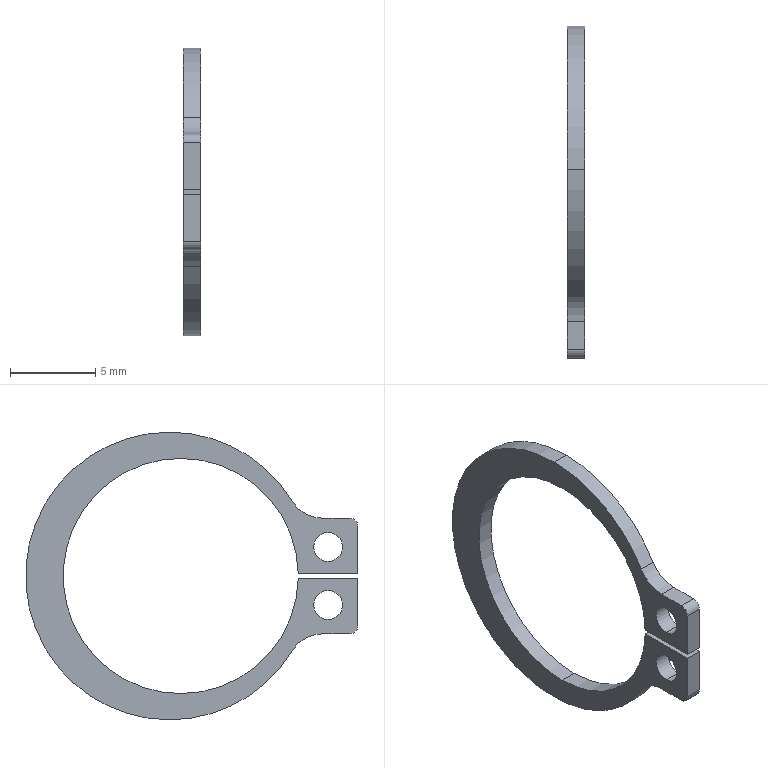Part | STEP file | 11-STWN1511 | 1 solid | 22 faces | box 1 x 19.5 x 16.88 mm | volume 88.469 mm3 | cylinder 14 | plane 8 | commonest cylinder face diameters 1.7 x4 13.8 x3 16.88 x3 1 x2 4 x2
STEP:
#1=CARTESIAN_POINT('',(0.5,-8.65,2.55));
#2=VERTEX_POINT('',#1);
#3=CARTESIAN_POINT('',(0.5,-8.65,0.85));
#4=VERTEX_POINT('',#3);
#5=CARTESIAN_POINT('',(0.5,-8.65,1.7));
#6=DIRECTION('',(1.,0.,0.));
#7=DIRECTION('',(0.,0.,-1.));
#8=AXIS2_PLACEMENT_3D('',#5,#6,#7);
#9=CIRCLE('',#8,0.85);
#10=EDGE_CURVE('',#2,#4,#9,.T.);
#11=ORIENTED_EDGE('',*,*,#10,.T.);
#12=CARTESIAN_POINT('',(-0.5,-8.65,0.85));
#13=VERTEX_POINT('',#12);
#14=CARTESIAN_POINT('',(0.5,-8.65,0.85));
#15=DIRECTION('',(-1.,0.,0.));
#16=VECTOR('',#15,1000.);
#17=LINE('',#14,#16);
#18=EDGE_CURVE('',#4,#13,#17,.T.);
#19=ORIENTED_EDGE('',*,*,#18,.T.);
#20=CARTESIAN_POINT('',(-0.5,-8.65,2.55));
#21=VERTEX_POINT('',#20);
#22=CARTESIAN_POINT('',(-0.5,-8.65,1.7));
#23=DIRECTION('',(1.,0.,0.));
#24=DIRECTION('',(0.,0.,-1.));
#25=AXIS2_PLACEMENT_3D('',#22,#23,#24);
#26=CIRCLE('',#25,0.85);
#27=EDGE_CURVE('',#21,#13,#26,.T.);
#28=ORIENTED_EDGE('',*,*,#27,.F.);
#29=CARTESIAN_POINT('',(0.5,-8.65,2.55));
#30=DIRECTION('',(-1.,0.,0.));
#31=VECTOR('',#30,1000.);
#32=LINE('',#29,#31);
#33=EDGE_CURVE('',#2,#21,#32,.T.);
#34=ORIENTED_EDGE('',*,*,#33,.F.);
#35=EDGE_LOOP('',(#11,#19,#28,#34));
#36=FACE_OUTER_BOUND('',#35,.T.);
#37=CARTESIAN_POINT('',(0.5,-8.65,1.7));
#38=DIRECTION('',(-1.,0.,0.));
#39=DIRECTION('',(0.,0.,1.));
#40=AXIS2_PLACEMENT_3D('',#37,#38,#39);
#41=CYLINDRICAL_SURFACE('',#40,0.85);
#42=ADVANCED_FACE('',(#36),#41,.F.);
#43=CARTESIAN_POINT('',(0.5,-8.65,-0.85));
#44=VERTEX_POINT('',#43);
#45=CARTESIAN_POINT('',(0.5,-8.65,-2.55));
#46=VERTEX_POINT('',#45);
#47=CARTESIAN_POINT('',(0.5,-8.65,-1.7));
#48=DIRECTION('',(1.,0.,0.));
#49=DIRECTION('',(0.,0.,-1.));
#50=AXIS2_PLACEMENT_3D('',#47,#48,#49);
#51=CIRCLE('',#50,0.85);
#52=EDGE_CURVE('',#44,#46,#51,.T.);
#53=ORIENTED_EDGE('',*,*,#52,.T.);
#54=CARTESIAN_POINT('',(-0.5,-8.65,-2.55));
#55=VERTEX_POINT('',#54);
#56=CARTESIAN_POINT('',(0.5,-8.65,-2.55));
#57=DIRECTION('',(-1.,0.,0.));
#58=VECTOR('',#57,1000.);
#59=LINE('',#56,#58);
#60=EDGE_CURVE('',#46,#55,#59,.T.);
#61=ORIENTED_EDGE('',*,*,#60,.T.);
#62=CARTESIAN_POINT('',(-0.5,-8.65,-0.85));
#63=VERTEX_POINT('',#62);
#64=CARTESIAN_POINT('',(-0.5,-8.65,-1.7));
#65=DIRECTION('',(1.,0.,0.));
#66=DIRECTION('',(0.,0.,-1.));
#67=AXIS2_PLACEMENT_3D('',#64,#65,#66);
#68=CIRCLE('',#67,0.85);
#69=EDGE_CURVE('',#63,#55,#68,.T.);
#70=ORIENTED_EDGE('',*,*,#69,.F.);
#71=CARTESIAN_POINT('',(0.5,-8.65,-0.85));
#72=DIRECTION('',(-1.,0.,0.));
#73=VECTOR('',#72,1000.);
#74=LINE('',#71,#73);
#75=EDGE_CURVE('',#44,#63,#74,.T.);
#76=ORIENTED_EDGE('',*,*,#75,.F.);
#77=EDGE_LOOP('',(#53,#61,#70,#76));
#78=FACE_OUTER_BOUND('',#77,.T.);
#79=CARTESIAN_POINT('',(0.5,-8.65,-1.7));
#80=DIRECTION('',(-1.,0.,0.));
#81=DIRECTION('',(0.,0.,1.));
#82=AXIS2_PLACEMENT_3D('',#79,#80,#81);
#83=CYLINDRICAL_SURFACE('',#82,0.85);
#84=ADVANCED_FACE('',(#78),#83,.F.);
#85=CARTESIAN_POINT('',(0.5,0.,-6.9));
#86=VERTEX_POINT('',#85);
#87=CARTESIAN_POINT('',(0.5,-6.899,-0.138));
#88=VERTEX_POINT('',#87);
#89=CARTESIAN_POINT('',(0.5,0.,0.));
#90=DIRECTION('',(-1.,0.,0.));
#91=DIRECTION('',(0.,0.,1.));
#92=AXIS2_PLACEMENT_3D('',#89,#90,#91);
#93=CIRCLE('',#92,6.9);
#94=EDGE_CURVE('',#86,#88,#93,.T.);
#95=ORIENTED_EDGE('',*,*,#94,.F.);
#96=CARTESIAN_POINT('',(-0.5,0.,-6.9));
#97=VERTEX_POINT('',#96);
#98=CARTESIAN_POINT('',(0.5,0.,-6.9));
#99=DIRECTION('',(-1.,0.,0.));
#100=VECTOR('',#99,1000.);
#101=LINE('',#98,#100);
#102=EDGE_CURVE('',#86,#97,#101,.T.);
#103=ORIENTED_EDGE('',*,*,#102,.T.);
#104=CARTESIAN_POINT('',(-0.5,-6.899,-0.138));
#105=VERTEX_POINT('',#104);
#106=CARTESIAN_POINT('',(-0.5,0.,0.));
#107=DIRECTION('',(-1.,0.,0.));
#108=DIRECTION('',(0.,0.,1.));
#109=AXIS2_PLACEMENT_3D('',#106,#107,#108);
#110=CIRCLE('',#109,6.9);
#111=EDGE_CURVE('',#97,#105,#110,.T.);
#112=ORIENTED_EDGE('',*,*,#111,.T.);
#113=CARTESIAN_POINT('',(0.5,-6.899,-0.138));
#114=DIRECTION('',(-1.,0.,0.));
#115=VECTOR('',#114,1000.);
#116=LINE('',#113,#115);
#117=EDGE_CURVE('',#88,#105,#116,.T.);
#118=ORIENTED_EDGE('',*,*,#117,.F.);
#119=EDGE_LOOP('',(#95,#103,#112,#118));
#120=FACE_OUTER_BOUND('',#119,.T.);
#121=CARTESIAN_POINT('',(0.5,0.,0.));
#122=DIRECTION('',(-1.,0.,0.));
#123=DIRECTION('',(0.,0.,1.));
#124=AXIS2_PLACEMENT_3D('',#121,#122,#123);
#125=CYLINDRICAL_SURFACE('',#124,6.9);
#126=ADVANCED_FACE('',(#120),#125,.F.);
#127=ORIENTED_EDGE('',*,*,#102,.F.);
#128=CARTESIAN_POINT('',(0.5,0.,6.9));
#129=VERTEX_POINT('',#128);
#130=CARTESIAN_POINT('',(0.5,0.,0.));
#131=DIRECTION('',(-1.,0.,0.));
#132=DIRECTION('',(0.,0.,1.));
#133=AXIS2_PLACEMENT_3D('',#130,#131,#132);
#134=CIRCLE('',#133,6.9);
#135=EDGE_CURVE('',#129,#86,#134,.T.);
#136=ORIENTED_EDGE('',*,*,#135,.F.);
#137=CARTESIAN_POINT('',(-0.5,0.,6.9));
#138=VERTEX_POINT('',#137);
#139=CARTESIAN_POINT('',(0.5,0.,6.9));
#140=DIRECTION('',(-1.,0.,0.));
#141=VECTOR('',#140,1000.);
#142=LINE('',#139,#141);
#143=EDGE_CURVE('',#129,#138,#142,.T.);
#144=ORIENTED_EDGE('',*,*,#143,.T.);
#145=CARTESIAN_POINT('',(-0.5,0.,0.));
#146=DIRECTION('',(-1.,0.,0.));
#147=DIRECTION('',(0.,0.,1.));
#148=AXIS2_PLACEMENT_3D('',#145,#146,#147);
#149=CIRCLE('',#148,6.9);
#150=EDGE_CURVE('',#138,#97,#149,.T.);
#151=ORIENTED_EDGE('',*,*,#150,.T.);
#152=EDGE_LOOP('',(#127,#136,#144,#151));
#153=FACE_OUTER_BOUND('',#152,.T.);
#154=CARTESIAN_POINT('',(0.5,0.,0.));
#155=DIRECTION('',(-1.,0.,0.));
#156=DIRECTION('',(0.,0.,1.));
#157=AXIS2_PLACEMENT_3D('',#154,#155,#156);
#158=CYLINDRICAL_SURFACE('',#157,6.9);
#159=ADVANCED_FACE('',(#153),#158,.F.);
#160=CARTESIAN_POINT('',(0.5,0.66,-8.44));
#161=VERTEX_POINT('',#160);
#162=CARTESIAN_POINT('',(0.5,0.66,8.44));
#163=VERTEX_POINT('',#162);
#164=CARTESIAN_POINT('',(0.5,0.66,0.));
#165=DIRECTION('',(1.,0.,0.));
#166=DIRECTION('',(0.,0.,-1.));
#167=AXIS2_PLACEMENT_3D('',#164,#165,#166);
#168=CIRCLE('',#167,8.44);
#169=EDGE_CURVE('',#161,#163,#168,.T.);
#170=ORIENTED_EDGE('',*,*,#169,.F.);
#171=CARTESIAN_POINT('',(-0.5,0.66,-8.44));
#172=VERTEX_POINT('',#171);
#173=CARTESIAN_POINT('',(0.5,0.66,-8.44));
#174=DIRECTION('',(-1.,0.,0.));
#175=VECTOR('',#174,1000.);
#176=LINE('',#173,#175);
#177=EDGE_CURVE('',#161,#172,#176,.T.);
#178=ORIENTED_EDGE('',*,*,#177,.T.);
#179=CARTESIAN_POINT('',(-0.5,0.66,8.44));
#180=VERTEX_POINT('',#179);
#181=CARTESIAN_POINT('',(-0.5,0.66,0.));
#182=DIRECTION('',(1.,0.,0.));
#183=DIRECTION('',(0.,0.,-1.));
#184=AXIS2_PLACEMENT_3D('',#181,#182,#183);
#185=CIRCLE('',#184,8.44);
#186=EDGE_CURVE('',#172,#180,#185,.T.);
#187=ORIENTED_EDGE('',*,*,#186,.T.);
#188=CARTESIAN_POINT('',(0.5,0.66,8.44));
#189=DIRECTION('',(-1.,0.,0.));
#190=VECTOR('',#189,1000.);
#191=LINE('',#188,#190);
#192=EDGE_CURVE('',#163,#180,#191,.T.);
#193=ORIENTED_EDGE('',*,*,#192,.F.);
#194=EDGE_LOOP('',(#170,#178,#187,#193));
#195=FACE_OUTER_BOUND('',#194,.T.);
#196=CARTESIAN_POINT('',(0.5,0.66,0.));
#197=DIRECTION('',(-1.,0.,0.));
#198=DIRECTION('',(0.,0.,1.));
#199=AXIS2_PLACEMENT_3D('',#196,#197,#198);
#200=CYLINDRICAL_SURFACE('',#199,8.44);
#201=ADVANCED_FACE('',(#195),#200,.T.);
#202=CARTESIAN_POINT('',(0.5,-6.563,4.366));
#203=VERTEX_POINT('',#202);
#204=CARTESIAN_POINT('',(0.5,0.66,0.));
#205=DIRECTION('',(1.,0.,0.));
#206=DIRECTION('',(0.,0.,-1.));
#207=AXIS2_PLACEMENT_3D('',#204,#205,#206);
#208=CIRCLE('',#207,8.44);
#209=EDGE_CURVE('',#163,#203,#208,.T.);
#210=ORIENTED_EDGE('',*,*,#209,.F.);
#211=ORIENTED_EDGE('',*,*,#192,.T.);
#212=CARTESIAN_POINT('',(-0.5,-6.563,4.366));
#213=VERTEX_POINT('',#212);
#214=CARTESIAN_POINT('',(-0.5,0.66,0.));
#215=DIRECTION('',(1.,0.,0.));
#216=DIRECTION('',(0.,0.,-1.));
#217=AXIS2_PLACEMENT_3D('',#214,#215,#216);
#218=CIRCLE('',#217,8.44);
#219=EDGE_CURVE('',#180,#213,#218,.T.);
#220=ORIENTED_EDGE('',*,*,#219,.T.);
#221=CARTESIAN_POINT('',(0.5,-6.563,4.366));
#222=DIRECTION('',(-1.,0.,0.));
#223=VECTOR('',#222,1000.);
#224=LINE('',#221,#223);
#225=EDGE_CURVE('',#203,#213,#224,.T.);
#226=ORIENTED_EDGE('',*,*,#225,.F.);
#227=EDGE_LOOP('',(#210,#211,#220,#226));
#228=FACE_OUTER_BOUND('',#227,.T.);
#229=CARTESIAN_POINT('',(0.5,0.66,0.));
#230=DIRECTION('',(-1.,0.,0.));
#231=DIRECTION('',(0.,0.,1.));
#232=AXIS2_PLACEMENT_3D('',#229,#230,#231);
#233=CYLINDRICAL_SURFACE('',#232,8.44);
#234=ADVANCED_FACE('',(#228),#233,.T.);
#235=ORIENTED_EDGE('',*,*,#52,.F.);
#236=CARTESIAN_POINT('',(0.5,-8.65,-1.7));
#237=DIRECTION('',(1.,0.,0.));
#238=DIRECTION('',(0.,0.,-1.));
#239=AXIS2_PLACEMENT_3D('',#236,#237,#238);
#240=CIRCLE('',#239,0.85);
#241=EDGE_CURVE('',#46,#44,#240,.T.);
#242=ORIENTED_EDGE('',*,*,#241,.F.);
#243=EDGE_LOOP('',(#235,#242));
#244=FACE_BOUND('',#243,.T.);
#245=CARTESIAN_POINT('',(0.5,-8.275,-3.4));
#246=VERTEX_POINT('',#245);
#247=CARTESIAN_POINT('',(0.5,-6.563,-4.366));
#248=VERTEX_POINT('',#247);
#249=CARTESIAN_POINT('',(0.5,-8.275,-5.4));
#250=DIRECTION('',(-1.,0.,0.));
#251=DIRECTION('',(0.,0.,1.));
#252=AXIS2_PLACEMENT_3D('',#249,#250,#251);
#253=CIRCLE('',#252,2.);
#254=EDGE_CURVE('',#246,#248,#253,.T.);
#255=ORIENTED_EDGE('',*,*,#254,.T.);
#256=CARTESIAN_POINT('',(0.5,0.66,0.));
#257=DIRECTION('',(1.,0.,0.));
#258=DIRECTION('',(0.,0.,-1.));
#259=AXIS2_PLACEMENT_3D('',#256,#257,#258);
#260=CIRCLE('',#259,8.44);
#261=EDGE_CURVE('',#248,#161,#260,.T.);
#262=ORIENTED_EDGE('',*,*,#261,.T.);
#263=ORIENTED_EDGE('',*,*,#169,.T.);
#264=ORIENTED_EDGE('',*,*,#209,.T.);
#265=CARTESIAN_POINT('',(0.5,-8.275,3.4));
#266=VERTEX_POINT('',#265);
#267=CARTESIAN_POINT('',(0.5,-8.275,5.4));
#268=DIRECTION('',(-1.,0.,0.));
#269=DIRECTION('',(0.,0.,1.));
#270=AXIS2_PLACEMENT_3D('',#267,#268,#269);
#271=CIRCLE('',#270,2.);
#272=EDGE_CURVE('',#203,#266,#271,.T.);
#273=ORIENTED_EDGE('',*,*,#272,.T.);
#274=CARTESIAN_POINT('',(0.5,-9.9,3.4));
#275=VERTEX_POINT('',#274);
#276=CARTESIAN_POINT('',(0.5,-8.275,3.4));
#277=DIRECTION('',(0.,-1.,0.));
#278=VECTOR('',#277,1000.);
#279=LINE('',#276,#278);
#280=EDGE_CURVE('',#266,#275,#279,.T.);
#281=ORIENTED_EDGE('',*,*,#280,.T.);
#282=CARTESIAN_POINT('',(0.5,-10.4,2.9));
#283=VERTEX_POINT('',#282);
#284=CARTESIAN_POINT('',(0.5,-9.9,2.9));
#285=DIRECTION('',(1.,0.,0.));
#286=DIRECTION('',(0.,0.,-1.));
#287=AXIS2_PLACEMENT_3D('',#284,#285,#286);
#288=CIRCLE('',#287,0.5);
#289=EDGE_CURVE('',#275,#283,#288,.T.);
#290=ORIENTED_EDGE('',*,*,#289,.T.);
#291=CARTESIAN_POINT('',(0.5,-10.4,0.138));
#292=VERTEX_POINT('',#291);
#293=CARTESIAN_POINT('',(0.5,-10.4,2.9));
#294=DIRECTION('',(0.,0.,-1.));
#295=VECTOR('',#294,1000.);
#296=LINE('',#293,#295);
#297=EDGE_CURVE('',#283,#292,#296,.T.);
#298=ORIENTED_EDGE('',*,*,#297,.T.);
#299=CARTESIAN_POINT('',(0.5,-6.899,0.138));
#300=VERTEX_POINT('',#299);
#301=CARTESIAN_POINT('',(0.5,-10.4,0.138));
#302=DIRECTION('',(0.,1.,0.));
#303=VECTOR('',#302,1000.);
#304=LINE('',#301,#303);
#305=EDGE_CURVE('',#292,#300,#304,.T.);
#306=ORIENTED_EDGE('',*,*,#305,.T.);
#307=CARTESIAN_POINT('',(0.5,0.,0.));
#308=DIRECTION('',(-1.,0.,0.));
#309=DIRECTION('',(0.,0.,1.));
#310=AXIS2_PLACEMENT_3D('',#307,#308,#309);
#311=CIRCLE('',#310,6.9);
#312=EDGE_CURVE('',#300,#129,#311,.T.);
#313=ORIENTED_EDGE('',*,*,#312,.T.);
#314=ORIENTED_EDGE('',*,*,#135,.T.);
#315=ORIENTED_EDGE('',*,*,#94,.T.);
#316=CARTESIAN_POINT('',(0.5,-10.4,-0.138));
#317=VERTEX_POINT('',#316);
#318=CARTESIAN_POINT('',(0.5,-6.899,-0.138));
#319=DIRECTION('',(0.,-1.,0.));
#320=VECTOR('',#319,1000.);
#321=LINE('',#318,#320);
#322=EDGE_CURVE('',#88,#317,#321,.T.);
#323=ORIENTED_EDGE('',*,*,#322,.T.);
#324=CARTESIAN_POINT('',(0.5,-10.4,-2.9));
#325=VERTEX_POINT('',#324);
#326=CARTESIAN_POINT('',(0.5,-10.4,-0.138));
#327=DIRECTION('',(0.,0.,-1.));
#328=VECTOR('',#327,1000.);
#329=LINE('',#326,#328);
#330=EDGE_CURVE('',#317,#325,#329,.T.);
#331=ORIENTED_EDGE('',*,*,#330,.T.);
#332=CARTESIAN_POINT('',(0.5,-9.9,-3.4));
#333=VERTEX_POINT('',#332);
#334=CARTESIAN_POINT('',(0.5,-9.9,-2.9));
#335=DIRECTION('',(1.,0.,0.));
#336=DIRECTION('',(0.,0.,-1.));
#337=AXIS2_PLACEMENT_3D('',#334,#335,#336);
#338=CIRCLE('',#337,0.5);
#339=EDGE_CURVE('',#325,#333,#338,.T.);
#340=ORIENTED_EDGE('',*,*,#339,.T.);
#341=CARTESIAN_POINT('',(0.5,-9.9,-3.4));
#342=DIRECTION('',(0.,1.,0.));
#343=VECTOR('',#342,1000.);
#344=LINE('',#341,#343);
#345=EDGE_CURVE('',#333,#246,#344,.T.);
#346=ORIENTED_EDGE('',*,*,#345,.T.);
#347=EDGE_LOOP('',(#255,#262,#263,#264,#273,#281,#290,#298,#306,#313,#314,#315,#323,#331,#340,#346));
#348=FACE_OUTER_BOUND('',#347,.T.);
#349=ORIENTED_EDGE('',*,*,#10,.F.);
#350=CARTESIAN_POINT('',(0.5,-8.65,1.7));
#351=DIRECTION('',(1.,0.,0.));
#352=DIRECTION('',(0.,0.,-1.));
#353=AXIS2_PLACEMENT_3D('',#350,#351,#352);
#354=CIRCLE('',#353,0.85);
#355=EDGE_CURVE('',#4,#2,#354,.T.);
#356=ORIENTED_EDGE('',*,*,#355,.F.);
#357=EDGE_LOOP('',(#349,#356));
#358=FACE_BOUND('',#357,.T.);
#359=CARTESIAN_POINT('',(0.5,-8.275,-5.4));
#360=DIRECTION('',(-1.,0.,0.));
#361=DIRECTION('',(0.,0.,1.));
#362=AXIS2_PLACEMENT_3D('',#359,#360,#361);
#363=PLANE('',#362);
#364=ADVANCED_FACE('',(#244,#348,#358),#363,.F.);
#365=CARTESIAN_POINT('',(-0.5,-8.275,-3.4));
#366=VERTEX_POINT('',#365);
#367=CARTESIAN_POINT('',(0.5,-8.275,-3.4));
#368=DIRECTION('',(-1.,0.,0.));
#369=VECTOR('',#368,1000.);
#370=LINE('',#367,#369);
#371=EDGE_CURVE('',#246,#366,#370,.T.);
#372=ORIENTED_EDGE('',*,*,#371,.T.);
#373=CARTESIAN_POINT('',(-0.5,-6.563,-4.366));
#374=VERTEX_POINT('',#373);
#375=CARTESIAN_POINT('',(-0.5,-8.275,-5.4));
#376=DIRECTION('',(-1.,0.,0.));
#377=DIRECTION('',(0.,0.,1.));
#378=AXIS2_PLACEMENT_3D('',#375,#376,#377);
#379=CIRCLE('',#378,2.);
#380=EDGE_CURVE('',#366,#374,#379,.T.);
#381=ORIENTED_EDGE('',*,*,#380,.T.);
#382=CARTESIAN_POINT('',(0.5,-6.563,-4.366));
#383=DIRECTION('',(-1.,0.,0.));
#384=VECTOR('',#383,1000.);
#385=LINE('',#382,#384);
#386=EDGE_CURVE('',#248,#374,#385,.T.);
#387=ORIENTED_EDGE('',*,*,#386,.F.);
#388=ORIENTED_EDGE('',*,*,#254,.F.);
#389=EDGE_LOOP('',(#372,#381,#387,#388));
#390=FACE_OUTER_BOUND('',#389,.T.);
#391=CARTESIAN_POINT('',(0.5,-8.275,-5.4));
#392=DIRECTION('',(-1.,0.,0.));
#393=DIRECTION('',(0.,0.,1.));
#394=AXIS2_PLACEMENT_3D('',#391,#392,#393);
#395=CYLINDRICAL_SURFACE('',#394,2.);
#396=ADVANCED_FACE('',(#390),#395,.F.);
#397=ORIENTED_EDGE('',*,*,#177,.F.);
#398=ORIENTED_EDGE('',*,*,#261,.F.);
#399=ORIENTED_EDGE('',*,*,#386,.T.);
#400=CARTESIAN_POINT('',(-0.5,0.66,0.));
#401=DIRECTION('',(1.,0.,0.));
#402=DIRECTION('',(0.,0.,-1.));
#403=AXIS2_PLACEMENT_3D('',#400,#401,#402);
#404=CIRCLE('',#403,8.44);
#405=EDGE_CURVE('',#374,#172,#404,.T.);
#406=ORIENTED_EDGE('',*,*,#405,.T.);
#407=EDGE_LOOP('',(#397,#398,#399,#406));
#408=FACE_OUTER_BOUND('',#407,.T.);
#409=CARTESIAN_POINT('',(0.5,0.66,0.));
#410=DIRECTION('',(-1.,0.,0.));
#411=DIRECTION('',(0.,0.,1.));
#412=AXIS2_PLACEMENT_3D('',#409,#410,#411);
#413=CYLINDRICAL_SURFACE('',#412,8.44);
#414=ADVANCED_FACE('',(#408),#413,.T.);
#415=ORIENTED_EDGE('',*,*,#225,.T.);
#416=CARTESIAN_POINT('',(-0.5,-8.275,3.4));
#417=VERTEX_POINT('',#416);
#418=CARTESIAN_POINT('',(-0.5,-8.275,5.4));
#419=DIRECTION('',(-1.,0.,0.));
#420=DIRECTION('',(0.,0.,1.));
#421=AXIS2_PLACEMENT_3D('',#418,#419,#420);
#422=CIRCLE('',#421,2.);
#423=EDGE_CURVE('',#213,#417,#422,.T.);
#424=ORIENTED_EDGE('',*,*,#423,.T.);
#425=CARTESIAN_POINT('',(0.5,-8.275,3.4));
#426=DIRECTION('',(-1.,0.,0.));
#427=VECTOR('',#426,1000.);
#428=LINE('',#425,#427);
#429=EDGE_CURVE('',#266,#417,#428,.T.);
#430=ORIENTED_EDGE('',*,*,#429,.F.);
#431=ORIENTED_EDGE('',*,*,#272,.F.);
#432=EDGE_LOOP('',(#415,#424,#430,#431));
#433=FACE_OUTER_BOUND('',#432,.T.);
#434=CARTESIAN_POINT('',(0.5,-8.275,5.4));
#435=DIRECTION('',(-1.,0.,0.));
#436=DIRECTION('',(0.,0.,1.));
#437=AXIS2_PLACEMENT_3D('',#434,#435,#436);
#438=CYLINDRICAL_SURFACE('',#437,2.);
#439=ADVANCED_FACE('',(#433),#438,.F.);
#440=ORIENTED_EDGE('',*,*,#429,.T.);
#441=CARTESIAN_POINT('',(-0.5,-9.9,3.4));
#442=VERTEX_POINT('',#441);
#443=CARTESIAN_POINT('',(-0.5,-8.275,3.4));
#444=DIRECTION('',(0.,-1.,0.));
#445=VECTOR('',#444,1000.);
#446=LINE('',#443,#445);
#447=EDGE_CURVE('',#417,#442,#446,.T.);
#448=ORIENTED_EDGE('',*,*,#447,.T.);
#449=CARTESIAN_POINT('',(0.5,-9.9,3.4));
#450=DIRECTION('',(-1.,0.,0.));
#451=VECTOR('',#450,1000.);
#452=LINE('',#449,#451);
#453=EDGE_CURVE('',#275,#442,#452,.T.);
#454=ORIENTED_EDGE('',*,*,#453,.F.);
#455=ORIENTED_EDGE('',*,*,#280,.F.);
#456=EDGE_LOOP('',(#440,#448,#454,#455));
#457=FACE_OUTER_BOUND('',#456,.T.);
#458=CARTESIAN_POINT('',(0.5,-8.275,3.4));
#459=DIRECTION('',(0.,0.,-1.));
#460=DIRECTION('',(-1.,0.,0.));
#461=AXIS2_PLACEMENT_3D('',#458,#459,#460);
#462=PLANE('',#461);
#463=ADVANCED_FACE('',(#457),#462,.F.);
#464=ORIENTED_EDGE('',*,*,#453,.T.);
#465=CARTESIAN_POINT('',(-0.5,-10.4,2.9));
#466=VERTEX_POINT('',#465);
#467=CARTESIAN_POINT('',(-0.5,-9.9,2.9));
#468=DIRECTION('',(1.,0.,0.));
#469=DIRECTION('',(0.,0.,-1.));
#470=AXIS2_PLACEMENT_3D('',#467,#468,#469);
#471=CIRCLE('',#470,0.5);
#472=EDGE_CURVE('',#442,#466,#471,.T.);
#473=ORIENTED_EDGE('',*,*,#472,.T.);
#474=CARTESIAN_POINT('',(0.5,-10.4,2.9));
#475=DIRECTION('',(-1.,0.,0.));
#476=VECTOR('',#475,1000.);
#477=LINE('',#474,#476);
#478=EDGE_CURVE('',#283,#466,#477,.T.);
#479=ORIENTED_EDGE('',*,*,#478,.F.);
#480=ORIENTED_EDGE('',*,*,#289,.F.);
#481=EDGE_LOOP('',(#464,#473,#479,#480));
#482=FACE_OUTER_BOUND('',#481,.T.);
#483=CARTESIAN_POINT('',(0.5,-9.9,2.9));
#484=DIRECTION('',(-1.,0.,0.));
#485=DIRECTION('',(0.,0.,1.));
#486=AXIS2_PLACEMENT_3D('',#483,#484,#485);
#487=CYLINDRICAL_SURFACE('',#486,0.5);
#488=ADVANCED_FACE('',(#482),#487,.T.);
#489=ORIENTED_EDGE('',*,*,#478,.T.);
#490=CARTESIAN_POINT('',(-0.5,-10.4,0.138));
#491=VERTEX_POINT('',#490);
#492=CARTESIAN_POINT('',(-0.5,-10.4,2.9));
#493=DIRECTION('',(0.,0.,-1.));
#494=VECTOR('',#493,1000.);
#495=LINE('',#492,#494);
#496=EDGE_CURVE('',#466,#491,#495,.T.);
#497=ORIENTED_EDGE('',*,*,#496,.T.);
#498=CARTESIAN_POINT('',(0.5,-10.4,0.138));
#499=DIRECTION('',(-1.,0.,0.));
#500=VECTOR('',#499,1000.);
#501=LINE('',#498,#500);
#502=EDGE_CURVE('',#292,#491,#501,.T.);
#503=ORIENTED_EDGE('',*,*,#502,.F.);
#504=ORIENTED_EDGE('',*,*,#297,.F.);
#505=EDGE_LOOP('',(#489,#497,#503,#504));
#506=FACE_OUTER_BOUND('',#505,.T.);
#507=CARTESIAN_POINT('',(0.5,-10.4,2.9));
#508=DIRECTION('',(0.,1.,0.));
#509=DIRECTION('',(0.,0.,1.));
#510=AXIS2_PLACEMENT_3D('',#507,#508,#509);
#511=PLANE('',#510);
#512=ADVANCED_FACE('',(#506),#511,.F.);
#513=ORIENTED_EDGE('',*,*,#502,.T.);
#514=CARTESIAN_POINT('',(-0.5,-6.899,0.138));
#515=VERTEX_POINT('',#514);
#516=CARTESIAN_POINT('',(-0.5,-10.4,0.138));
#517=DIRECTION('',(0.,1.,0.));
#518=VECTOR('',#517,1000.);
#519=LINE('',#516,#518);
#520=EDGE_CURVE('',#491,#515,#519,.T.);
#521=ORIENTED_EDGE('',*,*,#520,.T.);
#522=CARTESIAN_POINT('',(0.5,-6.899,0.138));
#523=DIRECTION('',(-1.,0.,0.));
#524=VECTOR('',#523,1000.);
#525=LINE('',#522,#524);
#526=EDGE_CURVE('',#300,#515,#525,.T.);
#527=ORIENTED_EDGE('',*,*,#526,.F.);
#528=ORIENTED_EDGE('',*,*,#305,.F.);
#529=EDGE_LOOP('',(#513,#521,#527,#528));
#530=FACE_OUTER_BOUND('',#529,.T.);
#531=CARTESIAN_POINT('',(0.5,-10.4,0.138));
#532=DIRECTION('',(0.,0.,1.));
#533=DIRECTION('',(1.,0.,0.));
#534=AXIS2_PLACEMENT_3D('',#531,#532,#533);
#535=PLANE('',#534);
#536=ADVANCED_FACE('',(#530),#535,.F.);
#537=ORIENTED_EDGE('',*,*,#143,.F.);
#538=ORIENTED_EDGE('',*,*,#312,.F.);
#539=ORIENTED_EDGE('',*,*,#526,.T.);
#540=CARTESIAN_POINT('',(-0.5,0.,0.));
#541=DIRECTION('',(-1.,0.,0.));
#542=DIRECTION('',(0.,0.,1.));
#543=AXIS2_PLACEMENT_3D('',#540,#541,#542);
#544=CIRCLE('',#543,6.9);
#545=EDGE_CURVE('',#515,#138,#544,.T.);
#546=ORIENTED_EDGE('',*,*,#545,.T.);
#547=EDGE_LOOP('',(#537,#538,#539,#546));
#548=FACE_OUTER_BOUND('',#547,.T.);
#549=CARTESIAN_POINT('',(0.5,0.,0.));
#550=DIRECTION('',(-1.,0.,0.));
#551=DIRECTION('',(0.,0.,1.));
#552=AXIS2_PLACEMENT_3D('',#549,#550,#551);
#553=CYLINDRICAL_SURFACE('',#552,6.9);
#554=ADVANCED_FACE('',(#548),#553,.F.);
#555=ORIENTED_EDGE('',*,*,#117,.T.);
#556=CARTESIAN_POINT('',(-0.5,-10.4,-0.138));
#557=VERTEX_POINT('',#556);
#558=CARTESIAN_POINT('',(-0.5,-6.899,-0.138));
#559=DIRECTION('',(0.,-1.,0.));
#560=VECTOR('',#559,1000.);
#561=LINE('',#558,#560);
#562=EDGE_CURVE('',#105,#557,#561,.T.);
#563=ORIENTED_EDGE('',*,*,#562,.T.);
#564=CARTESIAN_POINT('',(0.5,-10.4,-0.138));
#565=DIRECTION('',(-1.,0.,0.));
#566=VECTOR('',#565,1000.);
#567=LINE('',#564,#566);
#568=EDGE_CURVE('',#317,#557,#567,.T.);
#569=ORIENTED_EDGE('',*,*,#568,.F.);
#570=ORIENTED_EDGE('',*,*,#322,.F.);
#571=EDGE_LOOP('',(#555,#563,#569,#570));
#572=FACE_OUTER_BOUND('',#571,.T.);
#573=CARTESIAN_POINT('',(0.5,-6.899,-0.138));
#574=DIRECTION('',(0.,0.,-1.));
#575=DIRECTION('',(-1.,0.,0.));
#576=AXIS2_PLACEMENT_3D('',#573,#574,#575);
#577=PLANE('',#576);
#578=ADVANCED_FACE('',(#572),#577,.F.);
#579=ORIENTED_EDGE('',*,*,#568,.T.);
#580=CARTESIAN_POINT('',(-0.5,-10.4,-2.9));
#581=VERTEX_POINT('',#580);
#582=CARTESIAN_POINT('',(-0.5,-10.4,-0.138));
#583=DIRECTION('',(0.,0.,-1.));
#584=VECTOR('',#583,1000.);
#585=LINE('',#582,#584);
#586=EDGE_CURVE('',#557,#581,#585,.T.);
#587=ORIENTED_EDGE('',*,*,#586,.T.);
#588=CARTESIAN_POINT('',(0.5,-10.4,-2.9));
#589=DIRECTION('',(-1.,0.,0.));
#590=VECTOR('',#589,1000.);
#591=LINE('',#588,#590);
#592=EDGE_CURVE('',#325,#581,#591,.T.);
#593=ORIENTED_EDGE('',*,*,#592,.F.);
#594=ORIENTED_EDGE('',*,*,#330,.F.);
#595=EDGE_LOOP('',(#579,#587,#593,#594));
#596=FACE_OUTER_BOUND('',#595,.T.);
#597=CARTESIAN_POINT('',(0.5,-10.4,-0.138));
#598=DIRECTION('',(0.,1.,0.));
#599=DIRECTION('',(0.,0.,1.));
#600=AXIS2_PLACEMENT_3D('',#597,#598,#599);
#601=PLANE('',#600);
#602=ADVANCED_FACE('',(#596),#601,.F.);
#603=ORIENTED_EDGE('',*,*,#592,.T.);
#604=CARTESIAN_POINT('',(-0.5,-9.9,-3.4));
#605=VERTEX_POINT('',#604);
#606=CARTESIAN_POINT('',(-0.5,-9.9,-2.9));
#607=DIRECTION('',(1.,0.,0.));
#608=DIRECTION('',(0.,0.,-1.));
#609=AXIS2_PLACEMENT_3D('',#606,#607,#608);
#610=CIRCLE('',#609,0.5);
#611=EDGE_CURVE('',#581,#605,#610,.T.);
#612=ORIENTED_EDGE('',*,*,#611,.T.);
#613=CARTESIAN_POINT('',(0.5,-9.9,-3.4));
#614=DIRECTION('',(-1.,0.,0.));
#615=VECTOR('',#614,1000.);
#616=LINE('',#613,#615);
#617=EDGE_CURVE('',#333,#605,#616,.T.);
#618=ORIENTED_EDGE('',*,*,#617,.F.);
#619=ORIENTED_EDGE('',*,*,#339,.F.);
#620=EDGE_LOOP('',(#603,#612,#618,#619));
#621=FACE_OUTER_BOUND('',#620,.T.);
#622=CARTESIAN_POINT('',(0.5,-9.9,-2.9));
#623=DIRECTION('',(-1.,0.,0.));
#624=DIRECTION('',(0.,0.,1.));
#625=AXIS2_PLACEMENT_3D('',#622,#623,#624);
#626=CYLINDRICAL_SURFACE('',#625,0.5);
#627=ADVANCED_FACE('',(#621),#626,.T.);
#628=ORIENTED_EDGE('',*,*,#617,.T.);
#629=CARTESIAN_POINT('',(-0.5,-9.9,-3.4));
#630=DIRECTION('',(0.,1.,0.));
#631=VECTOR('',#630,1000.);
#632=LINE('',#629,#631);
#633=EDGE_CURVE('',#605,#366,#632,.T.);
#634=ORIENTED_EDGE('',*,*,#633,.T.);
#635=ORIENTED_EDGE('',*,*,#371,.F.);
#636=ORIENTED_EDGE('',*,*,#345,.F.);
#637=EDGE_LOOP('',(#628,#634,#635,#636));
#638=FACE_OUTER_BOUND('',#637,.T.);
#639=CARTESIAN_POINT('',(0.5,-9.9,-3.4));
#640=DIRECTION('',(0.,0.,1.));
#641=DIRECTION('',(1.,0.,0.));
#642=AXIS2_PLACEMENT_3D('',#639,#640,#641);
#643=PLANE('',#642);
#644=ADVANCED_FACE('',(#638),#643,.F.);
#645=ORIENTED_EDGE('',*,*,#60,.F.);
#646=ORIENTED_EDGE('',*,*,#241,.T.);
#647=ORIENTED_EDGE('',*,*,#75,.T.);
#648=CARTESIAN_POINT('',(-0.5,-8.65,-1.7));
#649=DIRECTION('',(1.,0.,0.));
#650=DIRECTION('',(0.,0.,-1.));
#651=AXIS2_PLACEMENT_3D('',#648,#649,#650);
#652=CIRCLE('',#651,0.85);
#653=EDGE_CURVE('',#55,#63,#652,.T.);
#654=ORIENTED_EDGE('',*,*,#653,.F.);
#655=EDGE_LOOP('',(#645,#646,#647,#654));
#656=FACE_OUTER_BOUND('',#655,.T.);
#657=CARTESIAN_POINT('',(0.5,-8.65,-1.7));
#658=DIRECTION('',(-1.,0.,0.));
#659=DIRECTION('',(0.,0.,1.));
#660=AXIS2_PLACEMENT_3D('',#657,#658,#659);
#661=CYLINDRICAL_SURFACE('',#660,0.85);
#662=ADVANCED_FACE('',(#656),#661,.F.);
#663=ORIENTED_EDGE('',*,*,#18,.F.);
#664=ORIENTED_EDGE('',*,*,#355,.T.);
#665=ORIENTED_EDGE('',*,*,#33,.T.);
#666=CARTESIAN_POINT('',(-0.5,-8.65,1.7));
#667=DIRECTION('',(1.,0.,0.));
#668=DIRECTION('',(0.,0.,-1.));
#669=AXIS2_PLACEMENT_3D('',#666,#667,#668);
#670=CIRCLE('',#669,0.85);
#671=EDGE_CURVE('',#13,#21,#670,.T.);
#672=ORIENTED_EDGE('',*,*,#671,.F.);
#673=EDGE_LOOP('',(#663,#664,#665,#672));
#674=FACE_OUTER_BOUND('',#673,.T.);
#675=CARTESIAN_POINT('',(0.5,-8.65,1.7));
#676=DIRECTION('',(-1.,0.,0.));
#677=DIRECTION('',(0.,0.,1.));
#678=AXIS2_PLACEMENT_3D('',#675,#676,#677);
#679=CYLINDRICAL_SURFACE('',#678,0.85);
#680=ADVANCED_FACE('',(#674),#679,.F.);
#681=ORIENTED_EDGE('',*,*,#27,.T.);
#682=ORIENTED_EDGE('',*,*,#671,.T.);
#683=EDGE_LOOP('',(#681,#682));
#684=FACE_BOUND('',#683,.T.);
#685=ORIENTED_EDGE('',*,*,#69,.T.);
#686=ORIENTED_EDGE('',*,*,#653,.T.);
#687=EDGE_LOOP('',(#685,#686));
#688=FACE_BOUND('',#687,.T.);
#689=ORIENTED_EDGE('',*,*,#380,.F.);
#690=ORIENTED_EDGE('',*,*,#633,.F.);
#691=ORIENTED_EDGE('',*,*,#611,.F.);
#692=ORIENTED_EDGE('',*,*,#586,.F.);
#693=ORIENTED_EDGE('',*,*,#562,.F.);
#694=ORIENTED_EDGE('',*,*,#111,.F.);
#695=ORIENTED_EDGE('',*,*,#150,.F.);
#696=ORIENTED_EDGE('',*,*,#545,.F.);
#697=ORIENTED_EDGE('',*,*,#520,.F.);
#698=ORIENTED_EDGE('',*,*,#496,.F.);
#699=ORIENTED_EDGE('',*,*,#472,.F.);
#700=ORIENTED_EDGE('',*,*,#447,.F.);
#701=ORIENTED_EDGE('',*,*,#423,.F.);
#702=ORIENTED_EDGE('',*,*,#219,.F.);
#703=ORIENTED_EDGE('',*,*,#186,.F.);
#704=ORIENTED_EDGE('',*,*,#405,.F.);
#705=EDGE_LOOP('',(#689,#690,#691,#692,#693,#694,#695,#696,#697,#698,#699,#700,#701,#702,#703,#704));
#706=FACE_OUTER_BOUND('',#705,.T.);
#707=CARTESIAN_POINT('',(-0.5,-8.275,-5.4));
#708=DIRECTION('',(-1.,0.,0.));
#709=DIRECTION('',(0.,0.,1.));
#710=AXIS2_PLACEMENT_3D('',#707,#708,#709);
#711=PLANE('',#710);
#712=ADVANCED_FACE('',(#684,#688,#706),#711,.T.);
#713=CLOSED_SHELL('',(#42,#84,#126,#159,#201,#234,#364,#396,#414,#439,#463,#488,#512,#536,#554,#578,#602,#627,#644,#662,#680,#712));
#714=MANIFOLD_SOLID_BREP('',#713);
#715=CARTESIAN_POINT('',(0.,0.,0.));
#716=DIRECTION('',(0.,0.,1.));
#717=DIRECTION('',(1.,0.,0.));
#718=AXIS2_PLACEMENT_3D('',#715,#716,#717);
#719=(LENGTH_UNIT()NAMED_UNIT(*)SI_UNIT(.MILLI.,.METRE.));
#720=UNCERTAINTY_MEASURE_WITH_UNIT(LENGTH_MEASURE(0.00001),#719,'','');
#721=(NAMED_UNIT(*)PLANE_ANGLE_UNIT()SI_UNIT($,.RADIAN.));
#722=(NAMED_UNIT(*)SI_UNIT($,.STERADIAN.)SOLID_ANGLE_UNIT());
#723=(GEOMETRIC_REPRESENTATION_CONTEXT(3)GLOBAL_UNCERTAINTY_ASSIGNED_CONTEXT((#720))GLOBAL_UNIT_ASSIGNED_CONTEXT((#719,#721,#722))REPRESENTATION_CONTEXT('',''));
#724=ADVANCED_BREP_SHAPE_REPRESENTATION('',(#714,#718),#723);